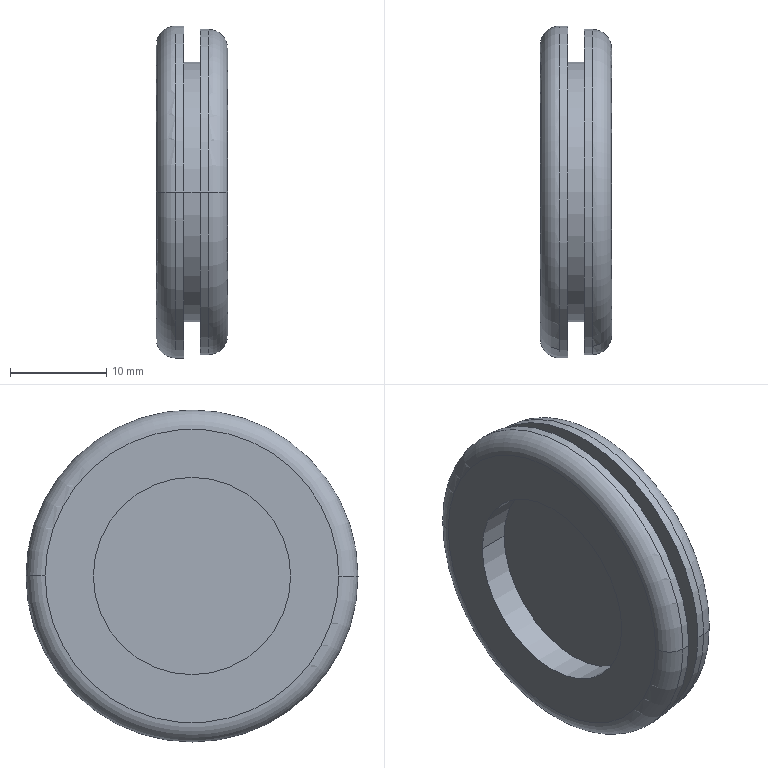Part | STEP file | 60008159 | 1 solid | 20 faces | box 7.4 x 34.5 x 34.5 mm | volume 3903 mm3 | cylinder 10 | plane 6 | torus 4 | commonest cylinder face diameters 20.5 x4 27 x2 33.8 x2 34.5 x2
STEP:
#1=CARTESIAN_POINT('',(0.,0.,0.));
#2=DIRECTION('',(0.,0.,1.));
#3=DIRECTION('',(1.,0.,0.));
#4=AXIS2_PLACEMENT_3D('',#1,#2,#3);
#5=CARTESIAN_POINT('',(-3.7,-15.25,0.));
#6=VERTEX_POINT('',#5);
#7=CARTESIAN_POINT('',(-3.7,15.25,0.));
#8=VERTEX_POINT('',#7);
#9=CARTESIAN_POINT('',(-3.7,0.,0.));
#10=DIRECTION('',(-1.,0.,0.));
#11=DIRECTION('',(0.,-1.,0.));
#12=AXIS2_PLACEMENT_3D('',#9,#10,#11);
#13=CIRCLE('',#12,15.25);
#14=CARTESIAN_POINT('',(-3.7,0.,0.));
#15=DIRECTION('',(1.,0.,0.));
#16=DIRECTION('',(0.,-1.,0.));
#17=AXIS2_PLACEMENT_3D('',#14,#15,#16);
#18=PLANE('',#17);
#19=CARTESIAN_POINT('',(15.25,0.));
#20=CARTESIAN_POINT('',(15.25,-26.414));
#21=CARTESIAN_POINT('',(-7.625,-13.207));
#22=CARTESIAN_POINT('',(-30.5,0.));
#23=CARTESIAN_POINT('',(-7.625,13.207));
#24=CARTESIAN_POINT('',(15.25,26.414));
#25=CARTESIAN_POINT('',(15.25,0.));
#26=(BOUNDED_CURVE()B_SPLINE_CURVE(2,(#19,#20,#21,#22,#23,#24,#25),.UNSPECIFIED.,.T.,.F.)B_SPLINE_CURVE_WITH_KNOTS((1,2,2,2,2,1),(-2.094,0.,2.094,4.189,6.283,8.378),.UNSPECIFIED.)CURVE()GEOMETRIC_REPRESENTATION_ITEM()RATIONAL_B_SPLINE_CURVE((1.,0.5,1.,0.5,1.,0.5,1.))REPRESENTATION_ITEM(''));
#27=(GEOMETRIC_REPRESENTATION_CONTEXT(2)PARAMETRIC_REPRESENTATION_CONTEXT()REPRESENTATION_CONTEXT('',''));
#28=DEFINITIONAL_REPRESENTATION('',(#26),#27);
#29=PCURVE('',#18,#28);
#30=CARTESIAN_POINT('',(-1.7,0.,0.));
#31=DIRECTION('',(1.,0.,0.));
#32=DIRECTION('',(0.,-1.,-0.00625));
#33=AXIS2_PLACEMENT_3D('',#30,#31,#32);
#34=TOROIDAL_SURFACE('',#33,15.25,2.);
#35=CARTESIAN_POINT('',(6.277,4.712));
#36=DIRECTION('',(-1.,0.));
#37=VECTOR('',#36,1.);
#38=LINE('',#35,#37);
#39=(GEOMETRIC_REPRESENTATION_CONTEXT(2)PARAMETRIC_REPRESENTATION_CONTEXT()REPRESENTATION_CONTEXT('',''));
#40=DEFINITIONAL_REPRESENTATION('',(#38),#39);
#41=PCURVE('',#34,#40);
#42=SURFACE_CURVE('',#13,(#29,#41),.PCURVE_S1.);
#43=EDGE_CURVE('',#6,#8,#42,.T.);
#44=ORIENTED_EDGE('',*,*,#43,.F.);
#45=CARTESIAN_POINT('',(-3.7,0.,0.));
#46=DIRECTION('',(-1.,0.,0.));
#47=DIRECTION('',(0.,1.,0.));
#48=AXIS2_PLACEMENT_3D('',#45,#46,#47);
#49=CIRCLE('',#48,15.25);
#50=CARTESIAN_POINT('',(-15.25,0.));
#51=CARTESIAN_POINT('',(-15.25,26.414));
#52=CARTESIAN_POINT('',(7.625,13.207));
#53=CARTESIAN_POINT('',(30.5,0.));
#54=CARTESIAN_POINT('',(7.625,-13.207));
#55=CARTESIAN_POINT('',(-15.25,-26.414));
#56=CARTESIAN_POINT('',(-15.25,0.));
#57=(BOUNDED_CURVE()B_SPLINE_CURVE(2,(#50,#51,#52,#53,#54,#55,#56),.UNSPECIFIED.,.T.,.F.)B_SPLINE_CURVE_WITH_KNOTS((1,2,2,2,2,1),(-2.094,0.,2.094,4.189,6.283,8.378),.UNSPECIFIED.)CURVE()GEOMETRIC_REPRESENTATION_ITEM()RATIONAL_B_SPLINE_CURVE((1.,0.5,1.,0.5,1.,0.5,1.))REPRESENTATION_ITEM(''));
#58=(GEOMETRIC_REPRESENTATION_CONTEXT(2)PARAMETRIC_REPRESENTATION_CONTEXT()REPRESENTATION_CONTEXT('',''));
#59=DEFINITIONAL_REPRESENTATION('',(#57),#58);
#60=PCURVE('',#18,#59);
#61=CARTESIAN_POINT('',(-1.7,0.,0.));
#62=DIRECTION('',(1.,0.,0.));
#63=DIRECTION('',(0.,1.,0.00625));
#64=AXIS2_PLACEMENT_3D('',#61,#62,#63);
#65=TOROIDAL_SURFACE('',#64,15.25,2.);
#66=CARTESIAN_POINT('',(6.277,4.712));
#67=DIRECTION('',(-1.,0.));
#68=VECTOR('',#67,1.);
#69=LINE('',#66,#68);
#70=(GEOMETRIC_REPRESENTATION_CONTEXT(2)PARAMETRIC_REPRESENTATION_CONTEXT()REPRESENTATION_CONTEXT('',''));
#71=DEFINITIONAL_REPRESENTATION('',(#69),#70);
#72=PCURVE('',#65,#71);
#73=SURFACE_CURVE('',#49,(#60,#72),.PCURVE_S1.);
#74=EDGE_CURVE('',#8,#6,#73,.T.);
#75=ORIENTED_EDGE('',*,*,#74,.F.);
#76=EDGE_LOOP('',(#44,#75));
#77=FACE_BOUND('',#76,.F.);
#78=CARTESIAN_POINT('',(-3.7,10.25,0.));
#79=VERTEX_POINT('',#78);
#80=CARTESIAN_POINT('',(-3.7,-10.25,0.));
#81=VERTEX_POINT('',#80);
#82=CARTESIAN_POINT('',(-3.7,0.,0.));
#83=DIRECTION('',(1.,0.,0.));
#84=DIRECTION('',(0.,1.,0.));
#85=AXIS2_PLACEMENT_3D('',#82,#83,#84);
#86=CIRCLE('',#85,10.25);
#87=CARTESIAN_POINT('',(0.,0.));
#88=DIRECTION('',(-1.,0.));
#89=AXIS2_PLACEMENT_2D('',#87,#88);
#90=CIRCLE('',#89,10.25);
#91=(GEOMETRIC_REPRESENTATION_CONTEXT(2)PARAMETRIC_REPRESENTATION_CONTEXT()REPRESENTATION_CONTEXT('',''));
#92=DEFINITIONAL_REPRESENTATION('',(#90),#91);
#93=PCURVE('',#18,#92);
#94=CARTESIAN_POINT('',(-4.07,0.,0.));
#95=DIRECTION('',(1.,0.,0.));
#96=DIRECTION('',(0.,-1.,0.));
#97=AXIS2_PLACEMENT_3D('',#94,#95,#96);
#98=CYLINDRICAL_SURFACE('',#97,10.25);
#99=CARTESIAN_POINT('',(3.142,0.37));
#100=DIRECTION('',(1.,0.));
#101=VECTOR('',#100,1.);
#102=LINE('',#99,#101);
#103=(GEOMETRIC_REPRESENTATION_CONTEXT(2)PARAMETRIC_REPRESENTATION_CONTEXT()REPRESENTATION_CONTEXT('',''));
#104=DEFINITIONAL_REPRESENTATION('',(#102),#103);
#105=PCURVE('',#98,#104);
#106=SURFACE_CURVE('',#86,(#93,#105),.PCURVE_S1.);
#107=EDGE_CURVE('',#79,#81,#106,.T.);
#108=ORIENTED_EDGE('',*,*,#107,.F.);
#109=CARTESIAN_POINT('',(-3.7,0.,0.));
#110=DIRECTION('',(-1.,0.,0.));
#111=DIRECTION('',(0.,1.,0.));
#112=AXIS2_PLACEMENT_3D('',#109,#110,#111);
#113=CIRCLE('',#112,10.25);
#114=CARTESIAN_POINT('',(-10.25,0.));
#115=CARTESIAN_POINT('',(-10.25,17.754));
#116=CARTESIAN_POINT('',(5.125,8.877));
#117=CARTESIAN_POINT('',(20.5,0.));
#118=CARTESIAN_POINT('',(5.125,-8.877));
#119=CARTESIAN_POINT('',(-10.25,-17.754));
#120=CARTESIAN_POINT('',(-10.25,0.));
#121=(BOUNDED_CURVE()B_SPLINE_CURVE(2,(#114,#115,#116,#117,#118,#119,#120),.UNSPECIFIED.,.T.,.F.)B_SPLINE_CURVE_WITH_KNOTS((1,2,2,2,2,1),(-2.094,0.,2.094,4.189,6.283,8.378),.UNSPECIFIED.)CURVE()GEOMETRIC_REPRESENTATION_ITEM()RATIONAL_B_SPLINE_CURVE((1.,0.5,1.,0.5,1.,0.5,1.))REPRESENTATION_ITEM(''));
#122=(GEOMETRIC_REPRESENTATION_CONTEXT(2)PARAMETRIC_REPRESENTATION_CONTEXT()REPRESENTATION_CONTEXT('',''));
#123=DEFINITIONAL_REPRESENTATION('',(#121),#122);
#124=PCURVE('',#18,#123);
#125=CARTESIAN_POINT('',(-4.07,0.,0.));
#126=DIRECTION('',(1.,0.,0.));
#127=DIRECTION('',(0.,-1.,0.));
#128=AXIS2_PLACEMENT_3D('',#125,#126,#127);
#129=CYLINDRICAL_SURFACE('',#128,10.25);
#130=CARTESIAN_POINT('',(3.142,0.37));
#131=DIRECTION('',(-1.,0.));
#132=VECTOR('',#131,1.);
#133=LINE('',#130,#132);
#134=(GEOMETRIC_REPRESENTATION_CONTEXT(2)PARAMETRIC_REPRESENTATION_CONTEXT()REPRESENTATION_CONTEXT('',''));
#135=DEFINITIONAL_REPRESENTATION('',(#133),#134);
#136=PCURVE('',#129,#135);
#137=SURFACE_CURVE('',#113,(#124,#136),.PCURVE_S1.);
#138=EDGE_CURVE('',#79,#81,#137,.T.);
#139=ORIENTED_EDGE('',*,*,#138,.T.);
#140=EDGE_LOOP('',(#108,#139));
#141=FACE_BOUND('',#140,.F.);
#142=ADVANCED_FACE('',(#77,#141),#18,.F.);
#143=CARTESIAN_POINT('',(-0.5,10.25,0.));
#144=VERTEX_POINT('',#143);
#145=CARTESIAN_POINT('',(-3.7,10.25,0.));
#146=DIRECTION('',(1.,0.,0.));
#147=VECTOR('',#146,1.);
#148=LINE('',#145,#147);
#149=CARTESIAN_POINT('',(3.142,0.37));
#150=DIRECTION('',(0.,1.));
#151=VECTOR('',#150,1.);
#152=LINE('',#149,#151);
#153=(GEOMETRIC_REPRESENTATION_CONTEXT(2)PARAMETRIC_REPRESENTATION_CONTEXT()REPRESENTATION_CONTEXT('',''));
#154=DEFINITIONAL_REPRESENTATION('',(#152),#153);
#155=PCURVE('',#98,#154);
#156=CARTESIAN_POINT('',(3.142,0.37));
#157=DIRECTION('',(0.,1.));
#158=VECTOR('',#157,1.);
#159=LINE('',#156,#158);
#160=(GEOMETRIC_REPRESENTATION_CONTEXT(2)PARAMETRIC_REPRESENTATION_CONTEXT()REPRESENTATION_CONTEXT('',''));
#161=DEFINITIONAL_REPRESENTATION('',(#159),#160);
#162=PCURVE('',#129,#161);
#163=SURFACE_CURVE('',#148,(#155,#162),.PCURVE_S1.);
#164=EDGE_CURVE('',#79,#144,#163,.T.);
#165=ORIENTED_EDGE('',*,*,#164,.F.);
#166=ORIENTED_EDGE('',*,*,#107,.T.);
#167=CARTESIAN_POINT('',(-0.5,-10.25,0.));
#168=VERTEX_POINT('',#167);
#169=CARTESIAN_POINT('',(-3.7,-10.25,0.));
#170=DIRECTION('',(1.,0.,0.));
#171=VECTOR('',#170,1.);
#172=LINE('',#169,#171);
#173=CARTESIAN_POINT('',(6.283,0.37));
#174=DIRECTION('',(0.,1.));
#175=VECTOR('',#174,1.);
#176=LINE('',#173,#175);
#177=(GEOMETRIC_REPRESENTATION_CONTEXT(2)PARAMETRIC_REPRESENTATION_CONTEXT()REPRESENTATION_CONTEXT('',''));
#178=DEFINITIONAL_REPRESENTATION('',(#176),#177);
#179=PCURVE('',#98,#178);
#180=CARTESIAN_POINT('',(0.,0.37));
#181=DIRECTION('',(0.,1.));
#182=VECTOR('',#181,1.);
#183=LINE('',#180,#182);
#184=(GEOMETRIC_REPRESENTATION_CONTEXT(2)PARAMETRIC_REPRESENTATION_CONTEXT()REPRESENTATION_CONTEXT('',''));
#185=DEFINITIONAL_REPRESENTATION('',(#183),#184);
#186=PCURVE('',#129,#185);
#187=SURFACE_CURVE('',#172,(#179,#186),.PCURVE_S1.);
#188=EDGE_CURVE('',#81,#168,#187,.T.);
#189=ORIENTED_EDGE('',*,*,#188,.T.);
#190=CARTESIAN_POINT('',(-0.5,0.,0.));
#191=DIRECTION('',(1.,0.,0.));
#192=DIRECTION('',(0.,1.,0.));
#193=AXIS2_PLACEMENT_3D('',#190,#191,#192);
#194=CIRCLE('',#193,10.25);
#195=CARTESIAN_POINT('',(3.142,3.57));
#196=DIRECTION('',(1.,0.));
#197=VECTOR('',#196,1.);
#198=LINE('',#195,#197);
#199=(GEOMETRIC_REPRESENTATION_CONTEXT(2)PARAMETRIC_REPRESENTATION_CONTEXT()REPRESENTATION_CONTEXT('',''));
#200=DEFINITIONAL_REPRESENTATION('',(#198),#199);
#201=PCURVE('',#98,#200);
#202=CARTESIAN_POINT('',(-0.5,0.,0.));
#203=DIRECTION('',(1.,0.,0.));
#204=DIRECTION('',(0.,-1.,0.));
#205=AXIS2_PLACEMENT_3D('',#202,#203,#204);
#206=PLANE('',#205);
#207=CARTESIAN_POINT('',(0.,0.));
#208=DIRECTION('',(-1.,0.));
#209=AXIS2_PLACEMENT_2D('',#207,#208);
#210=CIRCLE('',#209,10.25);
#211=(GEOMETRIC_REPRESENTATION_CONTEXT(2)PARAMETRIC_REPRESENTATION_CONTEXT()REPRESENTATION_CONTEXT('',''));
#212=DEFINITIONAL_REPRESENTATION('',(#210),#211);
#213=PCURVE('',#206,#212);
#214=SURFACE_CURVE('',#194,(#201,#213),.PCURVE_S1.);
#215=EDGE_CURVE('',#144,#168,#214,.T.);
#216=ORIENTED_EDGE('',*,*,#215,.F.);
#217=EDGE_LOOP('',(#165,#166,#189,#216));
#218=FACE_BOUND('',#217,.F.);
#219=ADVANCED_FACE('',(#218),#98,.F.);
#220=ORIENTED_EDGE('',*,*,#164,.T.);
#221=CARTESIAN_POINT('',(-0.5,0.,0.));
#222=DIRECTION('',(-1.,0.,0.));
#223=DIRECTION('',(0.,1.,0.));
#224=AXIS2_PLACEMENT_3D('',#221,#222,#223);
#225=CIRCLE('',#224,10.25);
#226=CARTESIAN_POINT('',(3.142,3.57));
#227=DIRECTION('',(-1.,0.));
#228=VECTOR('',#227,1.);
#229=LINE('',#226,#228);
#230=(GEOMETRIC_REPRESENTATION_CONTEXT(2)PARAMETRIC_REPRESENTATION_CONTEXT()REPRESENTATION_CONTEXT('',''));
#231=DEFINITIONAL_REPRESENTATION('',(#229),#230);
#232=PCURVE('',#129,#231);
#233=CARTESIAN_POINT('',(-10.25,0.));
#234=CARTESIAN_POINT('',(-10.25,17.754));
#235=CARTESIAN_POINT('',(5.125,8.877));
#236=CARTESIAN_POINT('',(20.5,0.));
#237=CARTESIAN_POINT('',(5.125,-8.877));
#238=CARTESIAN_POINT('',(-10.25,-17.754));
#239=CARTESIAN_POINT('',(-10.25,0.));
#240=(BOUNDED_CURVE()B_SPLINE_CURVE(2,(#233,#234,#235,#236,#237,#238,#239),.UNSPECIFIED.,.T.,.F.)B_SPLINE_CURVE_WITH_KNOTS((1,2,2,2,2,1),(-2.094,0.,2.094,4.189,6.283,8.378),.UNSPECIFIED.)CURVE()GEOMETRIC_REPRESENTATION_ITEM()RATIONAL_B_SPLINE_CURVE((1.,0.5,1.,0.5,1.,0.5,1.))REPRESENTATION_ITEM(''));
#241=(GEOMETRIC_REPRESENTATION_CONTEXT(2)PARAMETRIC_REPRESENTATION_CONTEXT()REPRESENTATION_CONTEXT('',''));
#242=DEFINITIONAL_REPRESENTATION('',(#240),#241);
#243=PCURVE('',#206,#242);
#244=SURFACE_CURVE('',#225,(#232,#243),.PCURVE_S1.);
#245=EDGE_CURVE('',#144,#168,#244,.T.);
#246=ORIENTED_EDGE('',*,*,#245,.T.);
#247=ORIENTED_EDGE('',*,*,#188,.F.);
#248=ORIENTED_EDGE('',*,*,#138,.F.);
#249=EDGE_LOOP('',(#220,#246,#247,#248));
#250=FACE_BOUND('',#249,.F.);
#251=ADVANCED_FACE('',(#250),#129,.F.);
#252=ORIENTED_EDGE('',*,*,#245,.F.);
#253=ORIENTED_EDGE('',*,*,#215,.T.);
#254=EDGE_LOOP('',(#252,#253));
#255=FACE_BOUND('',#254,.F.);
#256=ADVANCED_FACE('',(#255),#206,.F.);
#257=CARTESIAN_POINT('',(-1.7,-17.25,0.));
#258=VERTEX_POINT('',#257);
#259=CARTESIAN_POINT('',(-1.7,-15.25,0.));
#260=DIRECTION('',(0.,0.,1.));
#261=DIRECTION('',(-1.,0.,0.));
#262=AXIS2_PLACEMENT_3D('',#259,#260,#261);
#263=CIRCLE('',#262,2.);
#264=CARTESIAN_POINT('',(6.277,4.712));
#265=DIRECTION('',(0.,1.));
#266=VECTOR('',#265,1.);
#267=LINE('',#264,#266);
#268=(GEOMETRIC_REPRESENTATION_CONTEXT(2)PARAMETRIC_REPRESENTATION_CONTEXT()REPRESENTATION_CONTEXT('',''));
#269=DEFINITIONAL_REPRESENTATION('',(#267),#268);
#270=PCURVE('',#34,#269);
#271=CARTESIAN_POINT('',(3.135,4.712));
#272=DIRECTION('',(0.,1.));
#273=VECTOR('',#272,1.);
#274=LINE('',#271,#273);
#275=(GEOMETRIC_REPRESENTATION_CONTEXT(2)PARAMETRIC_REPRESENTATION_CONTEXT()REPRESENTATION_CONTEXT('',''));
#276=DEFINITIONAL_REPRESENTATION('',(#274),#275);
#277=PCURVE('',#65,#276);
#278=SURFACE_CURVE('',#263,(#270,#277),.PCURVE_S1.);
#279=EDGE_CURVE('',#6,#258,#278,.T.);
#280=ORIENTED_EDGE('',*,*,#279,.T.);
#281=CARTESIAN_POINT('',(-1.7,17.25,0.));
#282=VERTEX_POINT('',#281);
#283=CARTESIAN_POINT('',(-1.7,0.,0.));
#284=DIRECTION('',(-1.,0.,0.));
#285=DIRECTION('',(0.,-1.,0.));
#286=AXIS2_PLACEMENT_3D('',#283,#284,#285);
#287=CIRCLE('',#286,17.25);
#288=CARTESIAN_POINT('',(6.277,6.283));
#289=DIRECTION('',(-1.,0.));
#290=VECTOR('',#289,1.);
#291=LINE('',#288,#290);
#292=(GEOMETRIC_REPRESENTATION_CONTEXT(2)PARAMETRIC_REPRESENTATION_CONTEXT()REPRESENTATION_CONTEXT('',''));
#293=DEFINITIONAL_REPRESENTATION('',(#291),#292);
#294=PCURVE('',#34,#293);
#295=CARTESIAN_POINT('',(-4.07,0.,0.));
#296=DIRECTION('',(1.,0.,0.));
#297=DIRECTION('',(0.,-1.,0.));
#298=AXIS2_PLACEMENT_3D('',#295,#296,#297);
#299=CYLINDRICAL_SURFACE('',#298,17.25);
#300=CARTESIAN_POINT('',(6.283,2.37));
#301=DIRECTION('',(-1.,0.));
#302=VECTOR('',#301,1.);
#303=LINE('',#300,#302);
#304=(GEOMETRIC_REPRESENTATION_CONTEXT(2)PARAMETRIC_REPRESENTATION_CONTEXT()REPRESENTATION_CONTEXT('',''));
#305=DEFINITIONAL_REPRESENTATION('',(#303),#304);
#306=PCURVE('',#299,#305);
#307=SURFACE_CURVE('',#287,(#294,#306),.PCURVE_S1.);
#308=EDGE_CURVE('',#258,#282,#307,.T.);
#309=ORIENTED_EDGE('',*,*,#308,.T.);
#310=CARTESIAN_POINT('',(-1.7,15.25,0.));
#311=DIRECTION('',(0.,0.,-1.));
#312=DIRECTION('',(-1.,0.,0.));
#313=AXIS2_PLACEMENT_3D('',#310,#311,#312);
#314=CIRCLE('',#313,2.);
#315=CARTESIAN_POINT('',(3.135,4.712));
#316=DIRECTION('',(0.,1.));
#317=VECTOR('',#316,1.);
#318=LINE('',#315,#317);
#319=(GEOMETRIC_REPRESENTATION_CONTEXT(2)PARAMETRIC_REPRESENTATION_CONTEXT()REPRESENTATION_CONTEXT('',''));
#320=DEFINITIONAL_REPRESENTATION('',(#318),#319);
#321=PCURVE('',#34,#320);
#322=CARTESIAN_POINT('',(6.277,4.712));
#323=DIRECTION('',(0.,1.));
#324=VECTOR('',#323,1.);
#325=LINE('',#322,#324);
#326=(GEOMETRIC_REPRESENTATION_CONTEXT(2)PARAMETRIC_REPRESENTATION_CONTEXT()REPRESENTATION_CONTEXT('',''));
#327=DEFINITIONAL_REPRESENTATION('',(#325),#326);
#328=PCURVE('',#65,#327);
#329=SURFACE_CURVE('',#314,(#321,#328),.PCURVE_S1.);
#330=EDGE_CURVE('',#8,#282,#329,.T.);
#331=ORIENTED_EDGE('',*,*,#330,.F.);
#332=ORIENTED_EDGE('',*,*,#43,.F.);
#333=EDGE_LOOP('',(#280,#309,#331,#332));
#334=FACE_BOUND('',#333,.T.);
#335=ADVANCED_FACE('',(#334),#34,.T.);
#336=ORIENTED_EDGE('',*,*,#330,.T.);
#337=CARTESIAN_POINT('',(-1.7,0.,0.));
#338=DIRECTION('',(-1.,0.,0.));
#339=DIRECTION('',(0.,1.,0.));
#340=AXIS2_PLACEMENT_3D('',#337,#338,#339);
#341=CIRCLE('',#340,17.25);
#342=CARTESIAN_POINT('',(6.277,6.283));
#343=DIRECTION('',(-1.,0.));
#344=VECTOR('',#343,1.);
#345=LINE('',#342,#344);
#346=(GEOMETRIC_REPRESENTATION_CONTEXT(2)PARAMETRIC_REPRESENTATION_CONTEXT()REPRESENTATION_CONTEXT('',''));
#347=DEFINITIONAL_REPRESENTATION('',(#345),#346);
#348=PCURVE('',#65,#347);
#349=CARTESIAN_POINT('',(-4.07,0.,0.));
#350=DIRECTION('',(1.,0.,0.));
#351=DIRECTION('',(0.,-1.,0.));
#352=AXIS2_PLACEMENT_3D('',#349,#350,#351);
#353=CYLINDRICAL_SURFACE('',#352,17.25);
#354=CARTESIAN_POINT('',(3.142,2.37));
#355=DIRECTION('',(-1.,0.));
#356=VECTOR('',#355,1.);
#357=LINE('',#354,#356);
#358=(GEOMETRIC_REPRESENTATION_CONTEXT(2)PARAMETRIC_REPRESENTATION_CONTEXT()REPRESENTATION_CONTEXT('',''));
#359=DEFINITIONAL_REPRESENTATION('',(#357),#358);
#360=PCURVE('',#353,#359);
#361=SURFACE_CURVE('',#341,(#348,#360),.PCURVE_S1.);
#362=EDGE_CURVE('',#282,#258,#361,.T.);
#363=ORIENTED_EDGE('',*,*,#362,.T.);
#364=ORIENTED_EDGE('',*,*,#279,.F.);
#365=ORIENTED_EDGE('',*,*,#74,.F.);
#366=EDGE_LOOP('',(#336,#363,#364,#365));
#367=FACE_BOUND('',#366,.T.);
#368=ADVANCED_FACE('',(#367),#65,.T.);
#369=CARTESIAN_POINT('',(-0.85,17.25,0.));
#370=VERTEX_POINT('',#369);
#371=CARTESIAN_POINT('',(-0.85,17.25,0.));
#372=DIRECTION('',(-1.,0.,0.));
#373=VECTOR('',#372,1.);
#374=LINE('',#371,#373);
#375=CARTESIAN_POINT('',(3.142,3.22));
#376=DIRECTION('',(0.,-1.));
#377=VECTOR('',#376,1.);
#378=LINE('',#375,#377);
#379=(GEOMETRIC_REPRESENTATION_CONTEXT(2)PARAMETRIC_REPRESENTATION_CONTEXT()REPRESENTATION_CONTEXT('',''));
#380=DEFINITIONAL_REPRESENTATION('',(#378),#379);
#381=PCURVE('',#353,#380);
#382=CARTESIAN_POINT('',(3.142,3.22));
#383=DIRECTION('',(0.,-1.));
#384=VECTOR('',#383,1.);
#385=LINE('',#382,#384);
#386=(GEOMETRIC_REPRESENTATION_CONTEXT(2)PARAMETRIC_REPRESENTATION_CONTEXT()REPRESENTATION_CONTEXT('',''));
#387=DEFINITIONAL_REPRESENTATION('',(#385),#386);
#388=PCURVE('',#299,#387);
#389=SURFACE_CURVE('',#374,(#381,#388),.PCURVE_S1.);
#390=EDGE_CURVE('',#370,#282,#389,.T.);
#391=ORIENTED_EDGE('',*,*,#390,.F.);
#392=CARTESIAN_POINT('',(-0.85,-17.25,0.));
#393=VERTEX_POINT('',#392);
#394=CARTESIAN_POINT('',(-0.85,0.,0.));
#395=DIRECTION('',(-1.,0.,0.));
#396=DIRECTION('',(0.,1.,0.));
#397=AXIS2_PLACEMENT_3D('',#394,#395,#396);
#398=CIRCLE('',#397,17.25);
#399=CARTESIAN_POINT('',(3.142,3.22));
#400=DIRECTION('',(-1.,0.));
#401=VECTOR('',#400,1.);
#402=LINE('',#399,#401);
#403=(GEOMETRIC_REPRESENTATION_CONTEXT(2)PARAMETRIC_REPRESENTATION_CONTEXT()REPRESENTATION_CONTEXT('',''));
#404=DEFINITIONAL_REPRESENTATION('',(#402),#403);
#405=PCURVE('',#353,#404);
#406=CARTESIAN_POINT('',(-0.85,0.,0.));
#407=DIRECTION('',(1.,0.,0.));
#408=DIRECTION('',(0.,-1.,0.));
#409=AXIS2_PLACEMENT_3D('',#406,#407,#408);
#410=PLANE('',#409);
#411=CARTESIAN_POINT('',(-17.25,0.));
#412=CARTESIAN_POINT('',(-17.25,29.878));
#413=CARTESIAN_POINT('',(8.625,14.939));
#414=CARTESIAN_POINT('',(34.5,0.));
#415=CARTESIAN_POINT('',(8.625,-14.939));
#416=CARTESIAN_POINT('',(-17.25,-29.878));
#417=CARTESIAN_POINT('',(-17.25,0.));
#418=(BOUNDED_CURVE()B_SPLINE_CURVE(2,(#411,#412,#413,#414,#415,#416,#417),.UNSPECIFIED.,.T.,.F.)B_SPLINE_CURVE_WITH_KNOTS((1,2,2,2,2,1),(-2.094,0.,2.094,4.189,6.283,8.378),.UNSPECIFIED.)CURVE()GEOMETRIC_REPRESENTATION_ITEM()RATIONAL_B_SPLINE_CURVE((1.,0.5,1.,0.5,1.,0.5,1.))REPRESENTATION_ITEM(''));
#419=(GEOMETRIC_REPRESENTATION_CONTEXT(2)PARAMETRIC_REPRESENTATION_CONTEXT()REPRESENTATION_CONTEXT('',''));
#420=DEFINITIONAL_REPRESENTATION('',(#418),#419);
#421=PCURVE('',#410,#420);
#422=SURFACE_CURVE('',#398,(#405,#421),.PCURVE_S1.);
#423=EDGE_CURVE('',#370,#393,#422,.T.);
#424=ORIENTED_EDGE('',*,*,#423,.T.);
#425=CARTESIAN_POINT('',(-0.85,-17.25,0.));
#426=DIRECTION('',(-1.,0.,0.));
#427=VECTOR('',#426,1.);
#428=LINE('',#425,#427);
#429=CARTESIAN_POINT('',(0.,3.22));
#430=DIRECTION('',(0.,-1.));
#431=VECTOR('',#430,1.);
#432=LINE('',#429,#431);
#433=(GEOMETRIC_REPRESENTATION_CONTEXT(2)PARAMETRIC_REPRESENTATION_CONTEXT()REPRESENTATION_CONTEXT('',''));
#434=DEFINITIONAL_REPRESENTATION('',(#432),#433);
#435=PCURVE('',#353,#434);
#436=CARTESIAN_POINT('',(6.283,3.22));
#437=DIRECTION('',(0.,-1.));
#438=VECTOR('',#437,1.);
#439=LINE('',#436,#438);
#440=(GEOMETRIC_REPRESENTATION_CONTEXT(2)PARAMETRIC_REPRESENTATION_CONTEXT()REPRESENTATION_CONTEXT('',''));
#441=DEFINITIONAL_REPRESENTATION('',(#439),#440);
#442=PCURVE('',#299,#441);
#443=SURFACE_CURVE('',#428,(#435,#442),.PCURVE_S1.);
#444=EDGE_CURVE('',#393,#258,#443,.T.);
#445=ORIENTED_EDGE('',*,*,#444,.T.);
#446=ORIENTED_EDGE('',*,*,#362,.F.);
#447=EDGE_LOOP('',(#391,#424,#445,#446));
#448=FACE_BOUND('',#447,.T.);
#449=ADVANCED_FACE('',(#448),#353,.T.);
#450=ORIENTED_EDGE('',*,*,#444,.F.);
#451=CARTESIAN_POINT('',(-0.85,0.,0.));
#452=DIRECTION('',(1.,0.,0.));
#453=DIRECTION('',(0.,1.,0.));
#454=AXIS2_PLACEMENT_3D('',#451,#452,#453);
#455=CIRCLE('',#454,17.25);
#456=CARTESIAN_POINT('',(3.142,3.22));
#457=DIRECTION('',(1.,0.));
#458=VECTOR('',#457,1.);
#459=LINE('',#456,#458);
#460=(GEOMETRIC_REPRESENTATION_CONTEXT(2)PARAMETRIC_REPRESENTATION_CONTEXT()REPRESENTATION_CONTEXT('',''));
#461=DEFINITIONAL_REPRESENTATION('',(#459),#460);
#462=PCURVE('',#299,#461);
#463=CARTESIAN_POINT('',(0.,0.));
#464=DIRECTION('',(-1.,0.));
#465=AXIS2_PLACEMENT_2D('',#463,#464);
#466=CIRCLE('',#465,17.25);
#467=(GEOMETRIC_REPRESENTATION_CONTEXT(2)PARAMETRIC_REPRESENTATION_CONTEXT()REPRESENTATION_CONTEXT('',''));
#468=DEFINITIONAL_REPRESENTATION('',(#466),#467);
#469=PCURVE('',#410,#468);
#470=SURFACE_CURVE('',#455,(#462,#469),.PCURVE_S1.);
#471=EDGE_CURVE('',#370,#393,#470,.T.);
#472=ORIENTED_EDGE('',*,*,#471,.F.);
#473=ORIENTED_EDGE('',*,*,#390,.T.);
#474=ORIENTED_EDGE('',*,*,#308,.F.);
#475=EDGE_LOOP('',(#450,#472,#473,#474));
#476=FACE_BOUND('',#475,.T.);
#477=ADVANCED_FACE('',(#476),#299,.T.);
#478=ORIENTED_EDGE('',*,*,#423,.T.);
#479=ORIENTED_EDGE('',*,*,#471,.F.);
#480=EDGE_LOOP('',(#478,#479));
#481=FACE_BOUND('',#480,.F.);
#482=CARTESIAN_POINT('',(-0.85,13.5,0.));
#483=VERTEX_POINT('',#482);
#484=CARTESIAN_POINT('',(-0.85,-13.5,0.));
#485=VERTEX_POINT('',#484);
#486=CARTESIAN_POINT('',(-0.85,0.,0.));
#487=DIRECTION('',(1.,0.,0.));
#488=DIRECTION('',(0.,1.,0.));
#489=AXIS2_PLACEMENT_3D('',#486,#487,#488);
#490=CIRCLE('',#489,13.5);
#491=CARTESIAN_POINT('',(0.,0.));
#492=DIRECTION('',(-1.,0.));
#493=AXIS2_PLACEMENT_2D('',#491,#492);
#494=CIRCLE('',#493,13.5);
#495=(GEOMETRIC_REPRESENTATION_CONTEXT(2)PARAMETRIC_REPRESENTATION_CONTEXT()REPRESENTATION_CONTEXT('',''));
#496=DEFINITIONAL_REPRESENTATION('',(#494),#495);
#497=PCURVE('',#410,#496);
#498=CARTESIAN_POINT('',(-4.07,0.,0.));
#499=DIRECTION('',(1.,0.,0.));
#500=DIRECTION('',(0.,-1.,0.));
#501=AXIS2_PLACEMENT_3D('',#498,#499,#500);
#502=CYLINDRICAL_SURFACE('',#501,13.5);
#503=CARTESIAN_POINT('',(3.142,3.22));
#504=DIRECTION('',(1.,0.));
#505=VECTOR('',#504,1.);
#506=LINE('',#503,#505);
#507=(GEOMETRIC_REPRESENTATION_CONTEXT(2)PARAMETRIC_REPRESENTATION_CONTEXT()REPRESENTATION_CONTEXT('',''));
#508=DEFINITIONAL_REPRESENTATION('',(#506),#507);
#509=PCURVE('',#502,#508);
#510=SURFACE_CURVE('',#490,(#497,#509),.PCURVE_S1.);
#511=EDGE_CURVE('',#483,#485,#510,.T.);
#512=ORIENTED_EDGE('',*,*,#511,.T.);
#513=CARTESIAN_POINT('',(-0.85,0.,0.));
#514=DIRECTION('',(-1.,0.,0.));
#515=DIRECTION('',(0.,1.,0.));
#516=AXIS2_PLACEMENT_3D('',#513,#514,#515);
#517=CIRCLE('',#516,13.5);
#518=CARTESIAN_POINT('',(-13.5,0.));
#519=CARTESIAN_POINT('',(-13.5,23.383));
#520=CARTESIAN_POINT('',(6.75,11.691));
#521=CARTESIAN_POINT('',(27.,0.));
#522=CARTESIAN_POINT('',(6.75,-11.691));
#523=CARTESIAN_POINT('',(-13.5,-23.383));
#524=CARTESIAN_POINT('',(-13.5,0.));
#525=(BOUNDED_CURVE()B_SPLINE_CURVE(2,(#518,#519,#520,#521,#522,#523,#524),.UNSPECIFIED.,.T.,.F.)B_SPLINE_CURVE_WITH_KNOTS((1,2,2,2,2,1),(-2.094,0.,2.094,4.189,6.283,8.378),.UNSPECIFIED.)CURVE()GEOMETRIC_REPRESENTATION_ITEM()RATIONAL_B_SPLINE_CURVE((1.,0.5,1.,0.5,1.,0.5,1.))REPRESENTATION_ITEM(''));
#526=(GEOMETRIC_REPRESENTATION_CONTEXT(2)PARAMETRIC_REPRESENTATION_CONTEXT()REPRESENTATION_CONTEXT('',''));
#527=DEFINITIONAL_REPRESENTATION('',(#525),#526);
#528=PCURVE('',#410,#527);
#529=CARTESIAN_POINT('',(-4.07,0.,0.));
#530=DIRECTION('',(1.,0.,0.));
#531=DIRECTION('',(0.,-1.,0.));
#532=AXIS2_PLACEMENT_3D('',#529,#530,#531);
#533=CYLINDRICAL_SURFACE('',#532,13.5);
#534=CARTESIAN_POINT('',(3.142,3.22));
#535=DIRECTION('',(-1.,0.));
#536=VECTOR('',#535,1.);
#537=LINE('',#534,#536);
#538=(GEOMETRIC_REPRESENTATION_CONTEXT(2)PARAMETRIC_REPRESENTATION_CONTEXT()REPRESENTATION_CONTEXT('',''));
#539=DEFINITIONAL_REPRESENTATION('',(#537),#538);
#540=PCURVE('',#533,#539);
#541=SURFACE_CURVE('',#517,(#528,#540),.PCURVE_S1.);
#542=EDGE_CURVE('',#483,#485,#541,.T.);
#543=ORIENTED_EDGE('',*,*,#542,.F.);
#544=EDGE_LOOP('',(#512,#543));
#545=FACE_BOUND('',#544,.F.);
#546=ADVANCED_FACE('',(#481,#545),#410,.T.);
#547=ORIENTED_EDGE('',*,*,#511,.T.);
#548=CARTESIAN_POINT('',(0.85,-13.5,0.));
#549=VERTEX_POINT('',#548);
#550=CARTESIAN_POINT('',(0.85,-13.5,0.));
#551=DIRECTION('',(-1.,0.,0.));
#552=VECTOR('',#551,1.);
#553=LINE('',#550,#552);
#554=CARTESIAN_POINT('',(6.283,4.92));
#555=DIRECTION('',(0.,-1.));
#556=VECTOR('',#555,1.);
#557=LINE('',#554,#556);
#558=(GEOMETRIC_REPRESENTATION_CONTEXT(2)PARAMETRIC_REPRESENTATION_CONTEXT()REPRESENTATION_CONTEXT('',''));
#559=DEFINITIONAL_REPRESENTATION('',(#557),#558);
#560=PCURVE('',#502,#559);
#561=CARTESIAN_POINT('',(0.,4.92));
#562=DIRECTION('',(0.,-1.));
#563=VECTOR('',#562,1.);
#564=LINE('',#561,#563);
#565=(GEOMETRIC_REPRESENTATION_CONTEXT(2)PARAMETRIC_REPRESENTATION_CONTEXT()REPRESENTATION_CONTEXT('',''));
#566=DEFINITIONAL_REPRESENTATION('',(#564),#565);
#567=PCURVE('',#533,#566);
#568=SURFACE_CURVE('',#553,(#560,#567),.PCURVE_S1.);
#569=EDGE_CURVE('',#549,#485,#568,.T.);
#570=ORIENTED_EDGE('',*,*,#569,.F.);
#571=CARTESIAN_POINT('',(0.85,13.5,0.));
#572=VERTEX_POINT('',#571);
#573=CARTESIAN_POINT('',(0.85,0.,0.));
#574=DIRECTION('',(1.,0.,0.));
#575=DIRECTION('',(0.,1.,0.));
#576=AXIS2_PLACEMENT_3D('',#573,#574,#575);
#577=CIRCLE('',#576,13.5);
#578=CARTESIAN_POINT('',(3.142,4.92));
#579=DIRECTION('',(1.,0.));
#580=VECTOR('',#579,1.);
#581=LINE('',#578,#580);
#582=(GEOMETRIC_REPRESENTATION_CONTEXT(2)PARAMETRIC_REPRESENTATION_CONTEXT()REPRESENTATION_CONTEXT('',''));
#583=DEFINITIONAL_REPRESENTATION('',(#581),#582);
#584=PCURVE('',#502,#583);
#585=CARTESIAN_POINT('',(0.85,0.,0.));
#586=DIRECTION('',(1.,0.,0.));
#587=DIRECTION('',(0.,-1.,0.));
#588=AXIS2_PLACEMENT_3D('',#585,#586,#587);
#589=PLANE('',#588);
#590=CARTESIAN_POINT('',(0.,0.));
#591=DIRECTION('',(-1.,0.));
#592=AXIS2_PLACEMENT_2D('',#590,#591);
#593=CIRCLE('',#592,13.5);
#594=(GEOMETRIC_REPRESENTATION_CONTEXT(2)PARAMETRIC_REPRESENTATION_CONTEXT()REPRESENTATION_CONTEXT('',''));
#595=DEFINITIONAL_REPRESENTATION('',(#593),#594);
#596=PCURVE('',#589,#595);
#597=SURFACE_CURVE('',#577,(#584,#596),.PCURVE_S1.);
#598=EDGE_CURVE('',#572,#549,#597,.T.);
#599=ORIENTED_EDGE('',*,*,#598,.F.);
#600=CARTESIAN_POINT('',(0.85,13.5,0.));
#601=DIRECTION('',(-1.,0.,0.));
#602=VECTOR('',#601,1.);
#603=LINE('',#600,#602);
#604=CARTESIAN_POINT('',(3.142,4.92));
#605=DIRECTION('',(0.,-1.));
#606=VECTOR('',#605,1.);
#607=LINE('',#604,#606);
#608=(GEOMETRIC_REPRESENTATION_CONTEXT(2)PARAMETRIC_REPRESENTATION_CONTEXT()REPRESENTATION_CONTEXT('',''));
#609=DEFINITIONAL_REPRESENTATION('',(#607),#608);
#610=PCURVE('',#502,#609);
#611=CARTESIAN_POINT('',(3.142,4.92));
#612=DIRECTION('',(0.,-1.));
#613=VECTOR('',#612,1.);
#614=LINE('',#611,#613);
#615=(GEOMETRIC_REPRESENTATION_CONTEXT(2)PARAMETRIC_REPRESENTATION_CONTEXT()REPRESENTATION_CONTEXT('',''));
#616=DEFINITIONAL_REPRESENTATION('',(#614),#615);
#617=PCURVE('',#533,#616);
#618=SURFACE_CURVE('',#603,(#610,#617),.PCURVE_S1.);
#619=EDGE_CURVE('',#572,#483,#618,.T.);
#620=ORIENTED_EDGE('',*,*,#619,.T.);
#621=EDGE_LOOP('',(#547,#570,#599,#620));
#622=FACE_BOUND('',#621,.T.);
#623=ADVANCED_FACE('',(#622),#502,.T.);
#624=CARTESIAN_POINT('',(0.85,0.,0.));
#625=DIRECTION('',(-1.,0.,0.));
#626=DIRECTION('',(0.,1.,0.));
#627=AXIS2_PLACEMENT_3D('',#624,#625,#626);
#628=CIRCLE('',#627,13.5);
#629=CARTESIAN_POINT('',(3.142,4.92));
#630=DIRECTION('',(-1.,0.));
#631=VECTOR('',#630,1.);
#632=LINE('',#629,#631);
#633=(GEOMETRIC_REPRESENTATION_CONTEXT(2)PARAMETRIC_REPRESENTATION_CONTEXT()REPRESENTATION_CONTEXT('',''));
#634=DEFINITIONAL_REPRESENTATION('',(#632),#633);
#635=PCURVE('',#533,#634);
#636=CARTESIAN_POINT('',(-13.5,0.));
#637=CARTESIAN_POINT('',(-13.5,23.383));
#638=CARTESIAN_POINT('',(6.75,11.691));
#639=CARTESIAN_POINT('',(27.,0.));
#640=CARTESIAN_POINT('',(6.75,-11.691));
#641=CARTESIAN_POINT('',(-13.5,-23.383));
#642=CARTESIAN_POINT('',(-13.5,0.));
#643=(BOUNDED_CURVE()B_SPLINE_CURVE(2,(#636,#637,#638,#639,#640,#641,#642),.UNSPECIFIED.,.T.,.F.)B_SPLINE_CURVE_WITH_KNOTS((1,2,2,2,2,1),(-2.094,0.,2.094,4.189,6.283,8.378),.UNSPECIFIED.)CURVE()GEOMETRIC_REPRESENTATION_ITEM()RATIONAL_B_SPLINE_CURVE((1.,0.5,1.,0.5,1.,0.5,1.))REPRESENTATION_ITEM(''));
#644=(GEOMETRIC_REPRESENTATION_CONTEXT(2)PARAMETRIC_REPRESENTATION_CONTEXT()REPRESENTATION_CONTEXT('',''));
#645=DEFINITIONAL_REPRESENTATION('',(#643),#644);
#646=PCURVE('',#589,#645);
#647=SURFACE_CURVE('',#628,(#635,#646),.PCURVE_S1.);
#648=EDGE_CURVE('',#572,#549,#647,.T.);
#649=ORIENTED_EDGE('',*,*,#648,.T.);
#650=ORIENTED_EDGE('',*,*,#569,.T.);
#651=ORIENTED_EDGE('',*,*,#542,.F.);
#652=ORIENTED_EDGE('',*,*,#619,.F.);
#653=EDGE_LOOP('',(#649,#650,#651,#652));
#654=FACE_BOUND('',#653,.T.);
#655=ADVANCED_FACE('',(#654),#533,.T.);
#656=CARTESIAN_POINT('',(0.85,16.9,0.));
#657=VERTEX_POINT('',#656);
#658=CARTESIAN_POINT('',(0.85,-16.9,0.));
#659=VERTEX_POINT('',#658);
#660=CARTESIAN_POINT('',(0.85,0.,0.));
#661=DIRECTION('',(1.,0.,0.));
#662=DIRECTION('',(0.,1.,0.));
#663=AXIS2_PLACEMENT_3D('',#660,#661,#662);
#664=CIRCLE('',#663,16.9);
#665=CARTESIAN_POINT('',(0.,0.));
#666=DIRECTION('',(-1.,0.));
#667=AXIS2_PLACEMENT_2D('',#665,#666);
#668=CIRCLE('',#667,16.9);
#669=(GEOMETRIC_REPRESENTATION_CONTEXT(2)PARAMETRIC_REPRESENTATION_CONTEXT()REPRESENTATION_CONTEXT('',''));
#670=DEFINITIONAL_REPRESENTATION('',(#668),#669);
#671=PCURVE('',#589,#670);
#672=CARTESIAN_POINT('',(-4.07,0.,0.));
#673=DIRECTION('',(1.,0.,0.));
#674=DIRECTION('',(0.,-1.,0.));
#675=AXIS2_PLACEMENT_3D('',#672,#673,#674);
#676=CYLINDRICAL_SURFACE('',#675,16.9);
#677=CARTESIAN_POINT('',(3.142,4.92));
#678=DIRECTION('',(1.,0.));
#679=VECTOR('',#678,1.);
#680=LINE('',#677,#679);
#681=(GEOMETRIC_REPRESENTATION_CONTEXT(2)PARAMETRIC_REPRESENTATION_CONTEXT()REPRESENTATION_CONTEXT('',''));
#682=DEFINITIONAL_REPRESENTATION('',(#680),#681);
#683=PCURVE('',#676,#682);
#684=SURFACE_CURVE('',#664,(#671,#683),.PCURVE_S1.);
#685=EDGE_CURVE('',#657,#659,#684,.T.);
#686=ORIENTED_EDGE('',*,*,#685,.T.);
#687=CARTESIAN_POINT('',(0.85,0.,0.));
#688=DIRECTION('',(-1.,0.,0.));
#689=DIRECTION('',(0.,1.,0.));
#690=AXIS2_PLACEMENT_3D('',#687,#688,#689);
#691=CIRCLE('',#690,16.9);
#692=CARTESIAN_POINT('',(-16.9,0.));
#693=CARTESIAN_POINT('',(-16.9,29.272));
#694=CARTESIAN_POINT('',(8.45,14.636));
#695=CARTESIAN_POINT('',(33.8,0.));
#696=CARTESIAN_POINT('',(8.45,-14.636));
#697=CARTESIAN_POINT('',(-16.9,-29.272));
#698=CARTESIAN_POINT('',(-16.9,0.));
#699=(BOUNDED_CURVE()B_SPLINE_CURVE(2,(#692,#693,#694,#695,#696,#697,#698),.UNSPECIFIED.,.T.,.F.)B_SPLINE_CURVE_WITH_KNOTS((1,2,2,2,2,1),(-2.094,0.,2.094,4.189,6.283,8.378),.UNSPECIFIED.)CURVE()GEOMETRIC_REPRESENTATION_ITEM()RATIONAL_B_SPLINE_CURVE((1.,0.5,1.,0.5,1.,0.5,1.))REPRESENTATION_ITEM(''));
#700=(GEOMETRIC_REPRESENTATION_CONTEXT(2)PARAMETRIC_REPRESENTATION_CONTEXT()REPRESENTATION_CONTEXT('',''));
#701=DEFINITIONAL_REPRESENTATION('',(#699),#700);
#702=PCURVE('',#589,#701);
#703=CARTESIAN_POINT('',(-4.07,0.,0.));
#704=DIRECTION('',(1.,0.,0.));
#705=DIRECTION('',(0.,-1.,0.));
#706=AXIS2_PLACEMENT_3D('',#703,#704,#705);
#707=CYLINDRICAL_SURFACE('',#706,16.9);
#708=CARTESIAN_POINT('',(3.142,4.92));
#709=DIRECTION('',(-1.,0.));
#710=VECTOR('',#709,1.);
#711=LINE('',#708,#710);
#712=(GEOMETRIC_REPRESENTATION_CONTEXT(2)PARAMETRIC_REPRESENTATION_CONTEXT()REPRESENTATION_CONTEXT('',''));
#713=DEFINITIONAL_REPRESENTATION('',(#711),#712);
#714=PCURVE('',#707,#713);
#715=SURFACE_CURVE('',#691,(#702,#714),.PCURVE_S1.);
#716=EDGE_CURVE('',#657,#659,#715,.T.);
#717=ORIENTED_EDGE('',*,*,#716,.F.);
#718=EDGE_LOOP('',(#686,#717));
#719=FACE_BOUND('',#718,.F.);
#720=ORIENTED_EDGE('',*,*,#648,.T.);
#721=ORIENTED_EDGE('',*,*,#598,.F.);
#722=EDGE_LOOP('',(#720,#721));
#723=FACE_BOUND('',#722,.F.);
#724=ADVANCED_FACE('',(#719,#723),#589,.F.);
#725=CARTESIAN_POINT('',(1.7,16.9,0.));
#726=VERTEX_POINT('',#725);
#727=CARTESIAN_POINT('',(1.7,16.9,0.));
#728=DIRECTION('',(-1.,0.,0.));
#729=VECTOR('',#728,1.);
#730=LINE('',#727,#729);
#731=CARTESIAN_POINT('',(3.142,5.77));
#732=DIRECTION('',(0.,-1.));
#733=VECTOR('',#732,1.);
#734=LINE('',#731,#733);
#735=(GEOMETRIC_REPRESENTATION_CONTEXT(2)PARAMETRIC_REPRESENTATION_CONTEXT()REPRESENTATION_CONTEXT('',''));
#736=DEFINITIONAL_REPRESENTATION('',(#734),#735);
#737=PCURVE('',#676,#736);
#738=CARTESIAN_POINT('',(3.142,5.77));
#739=DIRECTION('',(0.,-1.));
#740=VECTOR('',#739,1.);
#741=LINE('',#738,#740);
#742=(GEOMETRIC_REPRESENTATION_CONTEXT(2)PARAMETRIC_REPRESENTATION_CONTEXT()REPRESENTATION_CONTEXT('',''));
#743=DEFINITIONAL_REPRESENTATION('',(#741),#742);
#744=PCURVE('',#707,#743);
#745=SURFACE_CURVE('',#730,(#737,#744),.PCURVE_S1.);
#746=EDGE_CURVE('',#726,#657,#745,.T.);
#747=ORIENTED_EDGE('',*,*,#746,.T.);
#748=ORIENTED_EDGE('',*,*,#685,.T.);
#749=CARTESIAN_POINT('',(1.7,-16.9,0.));
#750=VERTEX_POINT('',#749);
#751=CARTESIAN_POINT('',(1.7,-16.9,0.));
#752=DIRECTION('',(-1.,0.,0.));
#753=VECTOR('',#752,1.);
#754=LINE('',#751,#753);
#755=CARTESIAN_POINT('',(6.283,5.77));
#756=DIRECTION('',(0.,-1.));
#757=VECTOR('',#756,1.);
#758=LINE('',#755,#757);
#759=(GEOMETRIC_REPRESENTATION_CONTEXT(2)PARAMETRIC_REPRESENTATION_CONTEXT()REPRESENTATION_CONTEXT('',''));
#760=DEFINITIONAL_REPRESENTATION('',(#758),#759);
#761=PCURVE('',#676,#760);
#762=CARTESIAN_POINT('',(0.,5.77));
#763=CARTESIAN_POINT('',(0.,5.757));
#764=CARTESIAN_POINT('',(0.,5.731));
#765=CARTESIAN_POINT('',(0.,5.693));
#766=CARTESIAN_POINT('',(0.,5.654));
#767=CARTESIAN_POINT('',(0.,5.615));
#768=CARTESIAN_POINT('',(0.,5.577));
#769=CARTESIAN_POINT('',(0.,5.538));
#770=CARTESIAN_POINT('',(0.,5.5));
#771=CARTESIAN_POINT('',(0.,5.461));
#772=CARTESIAN_POINT('',(0.,5.422));
#773=CARTESIAN_POINT('',(0.,5.384));
#774=CARTESIAN_POINT('',(0.,5.345));
#775=CARTESIAN_POINT('',(0.,5.306));
#776=CARTESIAN_POINT('',(0.,5.268));
#777=CARTESIAN_POINT('',(0.,5.229));
#778=CARTESIAN_POINT('',(0.,5.19));
#779=CARTESIAN_POINT('',(0.,5.152));
#780=CARTESIAN_POINT('',(0.,5.113));
#781=CARTESIAN_POINT('',(0.,5.075));
#782=CARTESIAN_POINT('',(0.,5.036));
#783=CARTESIAN_POINT('',(0.,4.997));
#784=CARTESIAN_POINT('',(0.,4.959));
#785=CARTESIAN_POINT('',(0.,4.933));
#786=CARTESIAN_POINT('',(0.,4.92));
#787=B_SPLINE_CURVE_WITH_KNOTS('',3,(#762,#763,#764,#765,#766,#767,#768,#769,#770,#771,#772,#773,#774,#775,#776,#777,#778,#779,#780,#781,#782,#783,#784,#785,#786),.UNSPECIFIED.,.F.,.F.,(4,1,1,1,1,1,1,1,1,1,1,1,1,1,1,1,1,1,1,1,1,1,4),(0.,0.03864,0.07727,0.1159,0.1545,0.1932,0.2318,0.2705,0.3091,0.3477,0.3864,0.425,0.4636,0.5023,0.5409,0.5795,0.6182,0.6568,0.6955,0.7341,0.7727,0.8114,0.85),.QUASI_UNIFORM_KNOTS.);
#788=(GEOMETRIC_REPRESENTATION_CONTEXT(2)PARAMETRIC_REPRESENTATION_CONTEXT()REPRESENTATION_CONTEXT('',''));
#789=DEFINITIONAL_REPRESENTATION('',(#787),#788);
#790=PCURVE('',#707,#789);
#791=SURFACE_CURVE('',#754,(#761,#790),.PCURVE_S1.);
#792=EDGE_CURVE('',#750,#659,#791,.T.);
#793=ORIENTED_EDGE('',*,*,#792,.F.);
#794=CARTESIAN_POINT('',(1.7,0.,0.));
#795=DIRECTION('',(-1.,0.,0.));
#796=DIRECTION('',(0.,-1.,0.));
#797=AXIS2_PLACEMENT_3D('',#794,#795,#796);
#798=CIRCLE('',#797,16.9);
#799=CARTESIAN_POINT('',(6.283,5.77));
#800=DIRECTION('',(-1.,0.));
#801=VECTOR('',#800,1.);
#802=LINE('',#799,#801);
#803=(GEOMETRIC_REPRESENTATION_CONTEXT(2)PARAMETRIC_REPRESENTATION_CONTEXT()REPRESENTATION_CONTEXT('',''));
#804=DEFINITIONAL_REPRESENTATION('',(#802),#803);
#805=PCURVE('',#676,#804);
#806=CARTESIAN_POINT('',(1.7,0.,0.));
#807=DIRECTION('',(1.,0.,0.));
#808=DIRECTION('',(0.,-1.,-0.004318));
#809=AXIS2_PLACEMENT_3D('',#806,#807,#808);
#810=TOROIDAL_SURFACE('',#809,14.9,2.);
#811=CARTESIAN_POINT('',(6.279,0.));
#812=DIRECTION('',(-1.,0.));
#813=VECTOR('',#812,1.);
#814=LINE('',#811,#813);
#815=(GEOMETRIC_REPRESENTATION_CONTEXT(2)PARAMETRIC_REPRESENTATION_CONTEXT()REPRESENTATION_CONTEXT('',''));
#816=DEFINITIONAL_REPRESENTATION('',(#814),#815);
#817=PCURVE('',#810,#816);
#818=SURFACE_CURVE('',#798,(#805,#817),.PCURVE_S1.);
#819=EDGE_CURVE('',#750,#726,#818,.T.);
#820=ORIENTED_EDGE('',*,*,#819,.T.);
#821=EDGE_LOOP('',(#747,#748,#793,#820));
#822=FACE_BOUND('',#821,.T.);
#823=ADVANCED_FACE('',(#822),#676,.T.);
#824=CARTESIAN_POINT('',(3.7,-14.9,0.));
#825=VERTEX_POINT('',#824);
#826=CARTESIAN_POINT('',(1.7,-14.9,0.));
#827=DIRECTION('',(0.,0.,1.));
#828=DIRECTION('',(0.,-1.,0.));
#829=AXIS2_PLACEMENT_3D('',#826,#827,#828);
#830=CIRCLE('',#829,2.);
#831=CARTESIAN_POINT('',(6.279,0.));
#832=DIRECTION('',(0.,1.));
#833=VECTOR('',#832,1.);
#834=LINE('',#831,#833);
#835=(GEOMETRIC_REPRESENTATION_CONTEXT(2)PARAMETRIC_REPRESENTATION_CONTEXT()REPRESENTATION_CONTEXT('',''));
#836=DEFINITIONAL_REPRESENTATION('',(#834),#835);
#837=PCURVE('',#810,#836);
#838=CARTESIAN_POINT('',(1.7,0.,0.));
#839=DIRECTION('',(1.,0.,0.));
#840=DIRECTION('',(0.,1.,0.004318));
#841=AXIS2_PLACEMENT_3D('',#838,#839,#840);
#842=TOROIDAL_SURFACE('',#841,14.9,2.);
#843=CARTESIAN_POINT('',(3.137,0.));
#844=DIRECTION('',(0.,1.));
#845=VECTOR('',#844,1.);
#846=LINE('',#843,#845);
#847=(GEOMETRIC_REPRESENTATION_CONTEXT(2)PARAMETRIC_REPRESENTATION_CONTEXT()REPRESENTATION_CONTEXT('',''));
#848=DEFINITIONAL_REPRESENTATION('',(#846),#847);
#849=PCURVE('',#842,#848);
#850=SURFACE_CURVE('',#830,(#837,#849),.PCURVE_S1.);
#851=EDGE_CURVE('',#750,#825,#850,.T.);
#852=ORIENTED_EDGE('',*,*,#851,.T.);
#853=CARTESIAN_POINT('',(3.7,14.9,0.));
#854=VERTEX_POINT('',#853);
#855=CARTESIAN_POINT('',(3.7,0.,0.));
#856=DIRECTION('',(-1.,0.,0.));
#857=DIRECTION('',(0.,-1.,0.));
#858=AXIS2_PLACEMENT_3D('',#855,#856,#857);
#859=CIRCLE('',#858,14.9);
#860=CARTESIAN_POINT('',(6.279,1.571));
#861=DIRECTION('',(-1.,0.));
#862=VECTOR('',#861,1.);
#863=LINE('',#860,#862);
#864=(GEOMETRIC_REPRESENTATION_CONTEXT(2)PARAMETRIC_REPRESENTATION_CONTEXT()REPRESENTATION_CONTEXT('',''));
#865=DEFINITIONAL_REPRESENTATION('',(#863),#864);
#866=PCURVE('',#810,#865);
#867=CARTESIAN_POINT('',(3.7,0.,0.));
#868=DIRECTION('',(1.,0.,0.));
#869=DIRECTION('',(0.,-1.,0.));
#870=AXIS2_PLACEMENT_3D('',#867,#868,#869);
#871=PLANE('',#870);
#872=CARTESIAN_POINT('',(14.9,0.));
#873=CARTESIAN_POINT('',(14.9,-25.808));
#874=CARTESIAN_POINT('',(-7.45,-12.904));
#875=CARTESIAN_POINT('',(-29.8,0.));
#876=CARTESIAN_POINT('',(-7.45,12.904));
#877=CARTESIAN_POINT('',(14.9,25.808));
#878=CARTESIAN_POINT('',(14.9,0.));
#879=(BOUNDED_CURVE()B_SPLINE_CURVE(2,(#872,#873,#874,#875,#876,#877,#878),.UNSPECIFIED.,.T.,.F.)B_SPLINE_CURVE_WITH_KNOTS((1,2,2,2,2,1),(-2.094,0.,2.094,4.189,6.283,8.378),.UNSPECIFIED.)CURVE()GEOMETRIC_REPRESENTATION_ITEM()RATIONAL_B_SPLINE_CURVE((1.,0.5,1.,0.5,1.,0.5,1.))REPRESENTATION_ITEM(''));
#880=(GEOMETRIC_REPRESENTATION_CONTEXT(2)PARAMETRIC_REPRESENTATION_CONTEXT()REPRESENTATION_CONTEXT('',''));
#881=DEFINITIONAL_REPRESENTATION('',(#879),#880);
#882=PCURVE('',#871,#881);
#883=SURFACE_CURVE('',#859,(#866,#882),.PCURVE_S1.);
#884=EDGE_CURVE('',#825,#854,#883,.T.);
#885=ORIENTED_EDGE('',*,*,#884,.T.);
#886=CARTESIAN_POINT('',(1.7,14.9,0.));
#887=DIRECTION('',(0.,0.,-1.));
#888=DIRECTION('',(0.,1.,0.));
#889=AXIS2_PLACEMENT_3D('',#886,#887,#888);
#890=CIRCLE('',#889,2.);
#891=CARTESIAN_POINT('',(3.137,0.));
#892=DIRECTION('',(0.,1.));
#893=VECTOR('',#892,1.);
#894=LINE('',#891,#893);
#895=(GEOMETRIC_REPRESENTATION_CONTEXT(2)PARAMETRIC_REPRESENTATION_CONTEXT()REPRESENTATION_CONTEXT('',''));
#896=DEFINITIONAL_REPRESENTATION('',(#894),#895);
#897=PCURVE('',#810,#896);
#898=CARTESIAN_POINT('',(6.279,0.));
#899=DIRECTION('',(0.,1.));
#900=VECTOR('',#899,1.);
#901=LINE('',#898,#900);
#902=(GEOMETRIC_REPRESENTATION_CONTEXT(2)PARAMETRIC_REPRESENTATION_CONTEXT()REPRESENTATION_CONTEXT('',''));
#903=DEFINITIONAL_REPRESENTATION('',(#901),#902);
#904=PCURVE('',#842,#903);
#905=SURFACE_CURVE('',#890,(#897,#904),.PCURVE_S1.);
#906=EDGE_CURVE('',#726,#854,#905,.T.);
#907=ORIENTED_EDGE('',*,*,#906,.F.);
#908=ORIENTED_EDGE('',*,*,#819,.F.);
#909=EDGE_LOOP('',(#852,#885,#907,#908));
#910=FACE_BOUND('',#909,.T.);
#911=ADVANCED_FACE('',(#910),#810,.T.);
#912=ORIENTED_EDGE('',*,*,#906,.T.);
#913=CARTESIAN_POINT('',(3.7,0.,0.));
#914=DIRECTION('',(-1.,0.,0.));
#915=DIRECTION('',(0.,1.,0.));
#916=AXIS2_PLACEMENT_3D('',#913,#914,#915);
#917=CIRCLE('',#916,14.9);
#918=CARTESIAN_POINT('',(6.279,1.571));
#919=DIRECTION('',(-1.,0.));
#920=VECTOR('',#919,1.);
#921=LINE('',#918,#920);
#922=(GEOMETRIC_REPRESENTATION_CONTEXT(2)PARAMETRIC_REPRESENTATION_CONTEXT()REPRESENTATION_CONTEXT('',''));
#923=DEFINITIONAL_REPRESENTATION('',(#921),#922);
#924=PCURVE('',#842,#923);
#925=CARTESIAN_POINT('',(-14.9,0.));
#926=CARTESIAN_POINT('',(-14.9,25.808));
#927=CARTESIAN_POINT('',(7.45,12.904));
#928=CARTESIAN_POINT('',(29.8,0.));
#929=CARTESIAN_POINT('',(7.45,-12.904));
#930=CARTESIAN_POINT('',(-14.9,-25.808));
#931=CARTESIAN_POINT('',(-14.9,0.));
#932=(BOUNDED_CURVE()B_SPLINE_CURVE(2,(#925,#926,#927,#928,#929,#930,#931),.UNSPECIFIED.,.T.,.F.)B_SPLINE_CURVE_WITH_KNOTS((1,2,2,2,2,1),(-2.094,0.,2.094,4.189,6.283,8.378),.UNSPECIFIED.)CURVE()GEOMETRIC_REPRESENTATION_ITEM()RATIONAL_B_SPLINE_CURVE((1.,0.5,1.,0.5,1.,0.5,1.))REPRESENTATION_ITEM(''));
#933=(GEOMETRIC_REPRESENTATION_CONTEXT(2)PARAMETRIC_REPRESENTATION_CONTEXT()REPRESENTATION_CONTEXT('',''));
#934=DEFINITIONAL_REPRESENTATION('',(#932),#933);
#935=PCURVE('',#871,#934);
#936=SURFACE_CURVE('',#917,(#924,#935),.PCURVE_S1.);
#937=EDGE_CURVE('',#854,#825,#936,.T.);
#938=ORIENTED_EDGE('',*,*,#937,.T.);
#939=ORIENTED_EDGE('',*,*,#851,.F.);
#940=CARTESIAN_POINT('',(1.7,0.,0.));
#941=DIRECTION('',(-1.,0.,0.));
#942=DIRECTION('',(0.,1.,0.));
#943=AXIS2_PLACEMENT_3D('',#940,#941,#942);
#944=CIRCLE('',#943,16.9);
#945=CARTESIAN_POINT('',(6.279,0.));
#946=DIRECTION('',(-1.,0.));
#947=VECTOR('',#946,1.);
#948=LINE('',#945,#947);
#949=(GEOMETRIC_REPRESENTATION_CONTEXT(2)PARAMETRIC_REPRESENTATION_CONTEXT()REPRESENTATION_CONTEXT('',''));
#950=DEFINITIONAL_REPRESENTATION('',(#948),#949);
#951=PCURVE('',#842,#950);
#952=CARTESIAN_POINT('',(3.142,5.77));
#953=DIRECTION('',(-1.,0.));
#954=VECTOR('',#953,1.);
#955=LINE('',#952,#954);
#956=(GEOMETRIC_REPRESENTATION_CONTEXT(2)PARAMETRIC_REPRESENTATION_CONTEXT()REPRESENTATION_CONTEXT('',''));
#957=DEFINITIONAL_REPRESENTATION('',(#955),#956);
#958=PCURVE('',#707,#957);
#959=SURFACE_CURVE('',#944,(#951,#958),.PCURVE_S1.);
#960=EDGE_CURVE('',#726,#750,#959,.T.);
#961=ORIENTED_EDGE('',*,*,#960,.F.);
#962=EDGE_LOOP('',(#912,#938,#939,#961));
#963=FACE_BOUND('',#962,.T.);
#964=ADVANCED_FACE('',(#963),#842,.T.);
#965=ORIENTED_EDGE('',*,*,#792,.T.);
#966=ORIENTED_EDGE('',*,*,#716,.F.);
#967=ORIENTED_EDGE('',*,*,#746,.F.);
#968=ORIENTED_EDGE('',*,*,#960,.T.);
#969=EDGE_LOOP('',(#965,#966,#967,#968));
#970=FACE_BOUND('',#969,.T.);
#971=ADVANCED_FACE('',(#970),#707,.T.);
#972=ORIENTED_EDGE('',*,*,#937,.T.);
#973=ORIENTED_EDGE('',*,*,#884,.T.);
#974=EDGE_LOOP('',(#972,#973));
#975=FACE_BOUND('',#974,.F.);
#976=CARTESIAN_POINT('',(3.7,10.25,0.));
#977=VERTEX_POINT('',#976);
#978=CARTESIAN_POINT('',(3.7,-10.25,0.));
#979=VERTEX_POINT('',#978);
#980=CARTESIAN_POINT('',(3.7,0.,0.));
#981=DIRECTION('',(1.,0.,0.));
#982=DIRECTION('',(0.,1.,0.));
#983=AXIS2_PLACEMENT_3D('',#980,#981,#982);
#984=CIRCLE('',#983,10.25);
#985=CARTESIAN_POINT('',(0.,0.));
#986=DIRECTION('',(-1.,0.));
#987=AXIS2_PLACEMENT_2D('',#985,#986);
#988=CIRCLE('',#987,10.25);
#989=(GEOMETRIC_REPRESENTATION_CONTEXT(2)PARAMETRIC_REPRESENTATION_CONTEXT()REPRESENTATION_CONTEXT('',''));
#990=DEFINITIONAL_REPRESENTATION('',(#988),#989);
#991=PCURVE('',#871,#990);
#992=CARTESIAN_POINT('',(-4.07,0.,0.));
#993=DIRECTION('',(1.,0.,0.));
#994=DIRECTION('',(0.,-1.,0.));
#995=AXIS2_PLACEMENT_3D('',#992,#993,#994);
#996=CYLINDRICAL_SURFACE('',#995,10.25);
#997=CARTESIAN_POINT('',(3.142,7.77));
#998=DIRECTION('',(1.,0.));
#999=VECTOR('',#998,1.);
#1000=LINE('',#997,#999);
#1001=(GEOMETRIC_REPRESENTATION_CONTEXT(2)PARAMETRIC_REPRESENTATION_CONTEXT()REPRESENTATION_CONTEXT('',''));
#1002=DEFINITIONAL_REPRESENTATION('',(#1000),#1001);
#1003=PCURVE('',#996,#1002);
#1004=SURFACE_CURVE('',#984,(#991,#1003),.PCURVE_S1.);
#1005=EDGE_CURVE('',#977,#979,#1004,.T.);
#1006=ORIENTED_EDGE('',*,*,#1005,.T.);
#1007=CARTESIAN_POINT('',(3.7,0.,0.));
#1008=DIRECTION('',(-1.,0.,0.));
#1009=DIRECTION('',(0.,1.,0.));
#1010=AXIS2_PLACEMENT_3D('',#1007,#1008,#1009);
#1011=CIRCLE('',#1010,10.25);
#1012=CARTESIAN_POINT('',(-10.25,0.));
#1013=CARTESIAN_POINT('',(-10.25,17.754));
#1014=CARTESIAN_POINT('',(5.125,8.877));
#1015=CARTESIAN_POINT('',(20.5,0.));
#1016=CARTESIAN_POINT('',(5.125,-8.877));
#1017=CARTESIAN_POINT('',(-10.25,-17.754));
#1018=CARTESIAN_POINT('',(-10.25,0.));
#1019=(BOUNDED_CURVE()B_SPLINE_CURVE(2,(#1012,#1013,#1014,#1015,#1016,#1017,#1018),.UNSPECIFIED.,.T.,.F.)B_SPLINE_CURVE_WITH_KNOTS((1,2,2,2,2,1),(-2.094,0.,2.094,4.189,6.283,8.378),.UNSPECIFIED.)CURVE()GEOMETRIC_REPRESENTATION_ITEM()RATIONAL_B_SPLINE_CURVE((1.,0.5,1.,0.5,1.,0.5,1.))REPRESENTATION_ITEM(''));
#1020=(GEOMETRIC_REPRESENTATION_CONTEXT(2)PARAMETRIC_REPRESENTATION_CONTEXT()REPRESENTATION_CONTEXT('',''));
#1021=DEFINITIONAL_REPRESENTATION('',(#1019),#1020);
#1022=PCURVE('',#871,#1021);
#1023=CARTESIAN_POINT('',(-4.07,0.,0.));
#1024=DIRECTION('',(1.,0.,0.));
#1025=DIRECTION('',(0.,-1.,0.));
#1026=AXIS2_PLACEMENT_3D('',#1023,#1024,#1025);
#1027=CYLINDRICAL_SURFACE('',#1026,10.25);
#1028=CARTESIAN_POINT('',(3.142,7.77));
#1029=DIRECTION('',(-1.,0.));
#1030=VECTOR('',#1029,1.);
#1031=LINE('',#1028,#1030);
#1032=(GEOMETRIC_REPRESENTATION_CONTEXT(2)PARAMETRIC_REPRESENTATION_CONTEXT()REPRESENTATION_CONTEXT('',''));
#1033=DEFINITIONAL_REPRESENTATION('',(#1031),#1032);
#1034=PCURVE('',#1027,#1033);
#1035=SURFACE_CURVE('',#1011,(#1022,#1034),.PCURVE_S1.);
#1036=EDGE_CURVE('',#977,#979,#1035,.T.);
#1037=ORIENTED_EDGE('',*,*,#1036,.F.);
#1038=EDGE_LOOP('',(#1006,#1037));
#1039=FACE_BOUND('',#1038,.F.);
#1040=ADVANCED_FACE('',(#975,#1039),#871,.T.);
#1041=CARTESIAN_POINT('',(0.5,10.25,0.));
#1042=VERTEX_POINT('',#1041);
#1043=CARTESIAN_POINT('',(0.5,10.25,0.));
#1044=DIRECTION('',(1.,0.,0.));
#1045=VECTOR('',#1044,1.);
#1046=LINE('',#1043,#1045);
#1047=CARTESIAN_POINT('',(3.142,4.57));
#1048=DIRECTION('',(0.,1.));
#1049=VECTOR('',#1048,1.);
#1050=LINE('',#1047,#1049);
#1051=(GEOMETRIC_REPRESENTATION_CONTEXT(2)PARAMETRIC_REPRESENTATION_CONTEXT()REPRESENTATION_CONTEXT('',''));
#1052=DEFINITIONAL_REPRESENTATION('',(#1050),#1051);
#1053=PCURVE('',#996,#1052);
#1054=CARTESIAN_POINT('',(3.142,4.57));
#1055=DIRECTION('',(0.,1.));
#1056=VECTOR('',#1055,1.);
#1057=LINE('',#1054,#1056);
#1058=(GEOMETRIC_REPRESENTATION_CONTEXT(2)PARAMETRIC_REPRESENTATION_CONTEXT()REPRESENTATION_CONTEXT('',''));
#1059=DEFINITIONAL_REPRESENTATION('',(#1057),#1058);
#1060=PCURVE('',#1027,#1059);
#1061=SURFACE_CURVE('',#1046,(#1053,#1060),.PCURVE_S1.);
#1062=EDGE_CURVE('',#1042,#977,#1061,.T.);
#1063=ORIENTED_EDGE('',*,*,#1062,.F.);
#1064=CARTESIAN_POINT('',(0.5,-10.25,0.));
#1065=VERTEX_POINT('',#1064);
#1066=CARTESIAN_POINT('',(0.5,0.,0.));
#1067=DIRECTION('',(1.,0.,0.));
#1068=DIRECTION('',(0.,1.,0.));
#1069=AXIS2_PLACEMENT_3D('',#1066,#1067,#1068);
#1070=CIRCLE('',#1069,10.25);
#1071=CARTESIAN_POINT('',(3.142,4.57));
#1072=DIRECTION('',(1.,0.));
#1073=VECTOR('',#1072,1.);
#1074=LINE('',#1071,#1073);
#1075=(GEOMETRIC_REPRESENTATION_CONTEXT(2)PARAMETRIC_REPRESENTATION_CONTEXT()REPRESENTATION_CONTEXT('',''));
#1076=DEFINITIONAL_REPRESENTATION('',(#1074),#1075);
#1077=PCURVE('',#996,#1076);
#1078=CARTESIAN_POINT('',(0.5,0.,0.));
#1079=DIRECTION('',(1.,0.,0.));
#1080=DIRECTION('',(0.,-1.,0.));
#1081=AXIS2_PLACEMENT_3D('',#1078,#1079,#1080);
#1082=PLANE('',#1081);
#1083=CARTESIAN_POINT('',(0.,0.));
#1084=DIRECTION('',(-1.,0.));
#1085=AXIS2_PLACEMENT_2D('',#1083,#1084);
#1086=CIRCLE('',#1085,10.25);
#1087=(GEOMETRIC_REPRESENTATION_CONTEXT(2)PARAMETRIC_REPRESENTATION_CONTEXT()REPRESENTATION_CONTEXT('',''));
#1088=DEFINITIONAL_REPRESENTATION('',(#1086),#1087);
#1089=PCURVE('',#1082,#1088);
#1090=SURFACE_CURVE('',#1070,(#1077,#1089),.PCURVE_S1.);
#1091=EDGE_CURVE('',#1042,#1065,#1090,.T.);
#1092=ORIENTED_EDGE('',*,*,#1091,.T.);
#1093=CARTESIAN_POINT('',(0.5,-10.25,0.));
#1094=DIRECTION('',(1.,0.,0.));
#1095=VECTOR('',#1094,1.);
#1096=LINE('',#1093,#1095);
#1097=CARTESIAN_POINT('',(6.283,4.57));
#1098=DIRECTION('',(0.,1.));
#1099=VECTOR('',#1098,1.);
#1100=LINE('',#1097,#1099);
#1101=(GEOMETRIC_REPRESENTATION_CONTEXT(2)PARAMETRIC_REPRESENTATION_CONTEXT()REPRESENTATION_CONTEXT('',''));
#1102=DEFINITIONAL_REPRESENTATION('',(#1100),#1101);
#1103=PCURVE('',#996,#1102);
#1104=CARTESIAN_POINT('',(0.,4.57));
#1105=DIRECTION('',(0.,1.));
#1106=VECTOR('',#1105,1.);
#1107=LINE('',#1104,#1106);
#1108=(GEOMETRIC_REPRESENTATION_CONTEXT(2)PARAMETRIC_REPRESENTATION_CONTEXT()REPRESENTATION_CONTEXT('',''));
#1109=DEFINITIONAL_REPRESENTATION('',(#1107),#1108);
#1110=PCURVE('',#1027,#1109);
#1111=SURFACE_CURVE('',#1096,(#1103,#1110),.PCURVE_S1.);
#1112=EDGE_CURVE('',#1065,#979,#1111,.T.);
#1113=ORIENTED_EDGE('',*,*,#1112,.T.);
#1114=ORIENTED_EDGE('',*,*,#1005,.F.);
#1115=EDGE_LOOP('',(#1063,#1092,#1113,#1114));
#1116=FACE_BOUND('',#1115,.F.);
#1117=ADVANCED_FACE('',(#1116),#996,.F.);
#1118=ORIENTED_EDGE('',*,*,#1062,.T.);
#1119=ORIENTED_EDGE('',*,*,#1036,.T.);
#1120=ORIENTED_EDGE('',*,*,#1112,.F.);
#1121=CARTESIAN_POINT('',(0.5,0.,0.));
#1122=DIRECTION('',(-1.,0.,0.));
#1123=DIRECTION('',(0.,1.,0.));
#1124=AXIS2_PLACEMENT_3D('',#1121,#1122,#1123);
#1125=CIRCLE('',#1124,10.25);
#1126=CARTESIAN_POINT('',(3.142,4.57));
#1127=DIRECTION('',(-1.,0.));
#1128=VECTOR('',#1127,1.);
#1129=LINE('',#1126,#1128);
#1130=(GEOMETRIC_REPRESENTATION_CONTEXT(2)PARAMETRIC_REPRESENTATION_CONTEXT()REPRESENTATION_CONTEXT('',''));
#1131=DEFINITIONAL_REPRESENTATION('',(#1129),#1130);
#1132=PCURVE('',#1027,#1131);
#1133=CARTESIAN_POINT('',(-10.25,0.));
#1134=CARTESIAN_POINT('',(-10.25,17.754));
#1135=CARTESIAN_POINT('',(5.125,8.877));
#1136=CARTESIAN_POINT('',(20.5,0.));
#1137=CARTESIAN_POINT('',(5.125,-8.877));
#1138=CARTESIAN_POINT('',(-10.25,-17.754));
#1139=CARTESIAN_POINT('',(-10.25,0.));
#1140=(BOUNDED_CURVE()B_SPLINE_CURVE(2,(#1133,#1134,#1135,#1136,#1137,#1138,#1139),.UNSPECIFIED.,.T.,.F.)B_SPLINE_CURVE_WITH_KNOTS((1,2,2,2,2,1),(-2.094,0.,2.094,4.189,6.283,8.378),.UNSPECIFIED.)CURVE()GEOMETRIC_REPRESENTATION_ITEM()RATIONAL_B_SPLINE_CURVE((1.,0.5,1.,0.5,1.,0.5,1.))REPRESENTATION_ITEM(''));
#1141=(GEOMETRIC_REPRESENTATION_CONTEXT(2)PARAMETRIC_REPRESENTATION_CONTEXT()REPRESENTATION_CONTEXT('',''));
#1142=DEFINITIONAL_REPRESENTATION('',(#1140),#1141);
#1143=PCURVE('',#1082,#1142);
#1144=SURFACE_CURVE('',#1125,(#1132,#1143),.PCURVE_S1.);
#1145=EDGE_CURVE('',#1042,#1065,#1144,.T.);
#1146=ORIENTED_EDGE('',*,*,#1145,.F.);
#1147=EDGE_LOOP('',(#1118,#1119,#1120,#1146));
#1148=FACE_BOUND('',#1147,.F.);
#1149=ADVANCED_FACE('',(#1148),#1027,.F.);
#1150=ORIENTED_EDGE('',*,*,#1145,.T.);
#1151=ORIENTED_EDGE('',*,*,#1091,.F.);
#1152=EDGE_LOOP('',(#1150,#1151));
#1153=FACE_BOUND('',#1152,.F.);
#1154=ADVANCED_FACE('',(#1153),#1082,.T.);
#1155=CLOSED_SHELL('',(#142,#219,#251,#256,#335,#368,#449,#477,#546,#623,#655,#724,#823,#911,#964,#971,#1040,#1117,#1149,#1154));
#1156=MANIFOLD_SOLID_BREP('',#1155);
#1157=(LENGTH_UNIT()NAMED_UNIT(*)SI_UNIT(.MILLI.,.METRE.));
#1158=UNCERTAINTY_MEASURE_WITH_UNIT(LENGTH_MEASURE(0.0000001),#1157,'','');
#1159=(NAMED_UNIT(*)PLANE_ANGLE_UNIT()SI_UNIT($,.RADIAN.));
#1160=(NAMED_UNIT(*)SI_UNIT($,.STERADIAN.)SOLID_ANGLE_UNIT());
#1161=(GEOMETRIC_REPRESENTATION_CONTEXT(3)GLOBAL_UNCERTAINTY_ASSIGNED_CONTEXT((#1158))GLOBAL_UNIT_ASSIGNED_CONTEXT((#1157,#1159,#1160))REPRESENTATION_CONTEXT('',''));
#1162=ADVANCED_BREP_SHAPE_REPRESENTATION('',(#4,#1156),#1161);